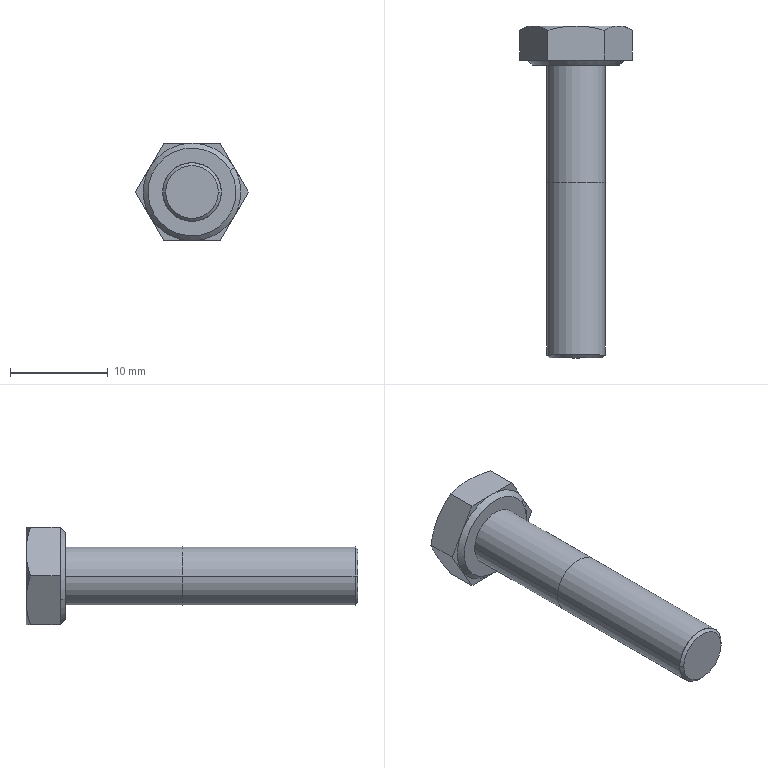Part | NX | features BREP 2 | 1 solid | 31 faces | box 11.547 x 34 x 10 mm | volume 1354 mm3 | plane 17 | cone 10 | cylinder 4 | commonest cylinder face diameters 4.917 x2 6 x2